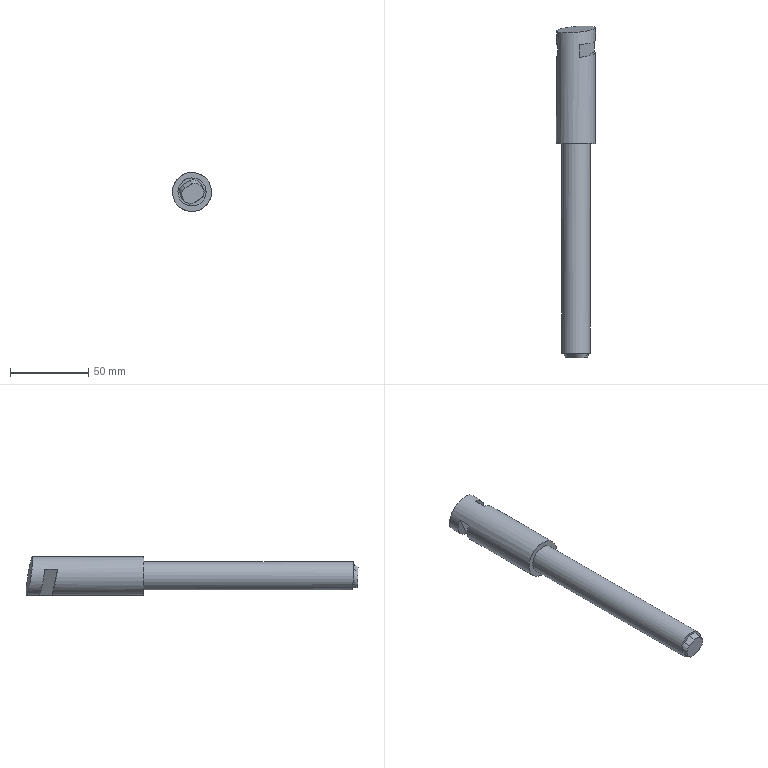Part | STEP file | solid 154 | 1 solid | 20 faces | box 25 x 212.652 x 25 mm | volume 69526 mm3 | spline 10 | plane 8 | cylinder 2 | commonest cylinder face diameters 18 x1 25 x1